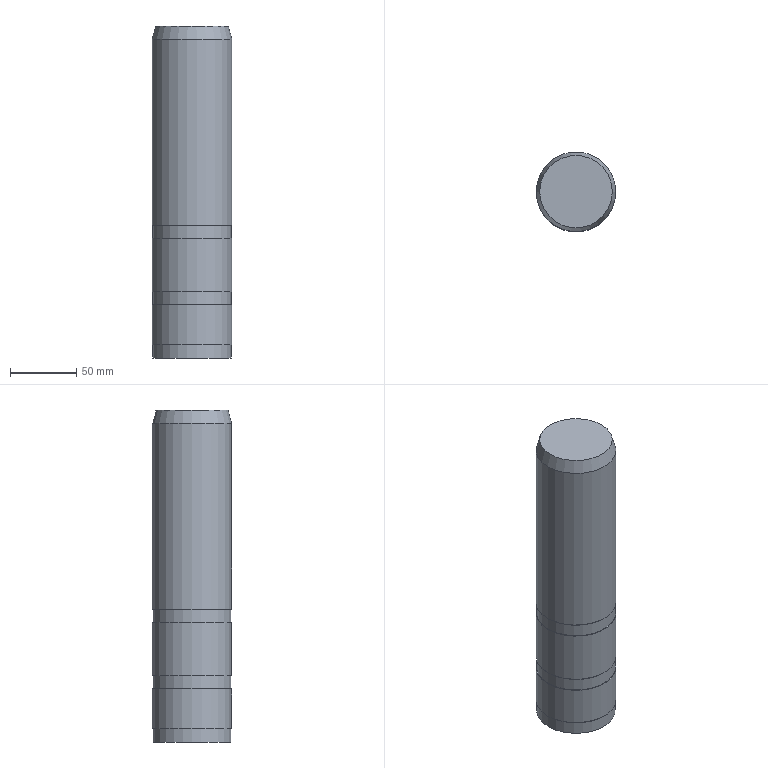Part | NX | features solid 2 | 1 solid | 14 faces | box 60 x 60 x 250 mm | volume 701604 mm3 | plane 7 | cylinder 6 | cone 1 | commonest cylinder face diameters 59 x3 60 x3
STEP:
#1=CARTESIAN_POINT('',(700.5,-25.,-150.));
#2=VERTEX_POINT('',#1);
#3=CARTESIAN_POINT('',(730.,-25.,-150.));
#4=DIRECTION('',(0.,0.,-1.));
#5=DIRECTION('',(-1.,0.,0.));
#6=AXIS2_PLACEMENT_3D('',#3,#4,#5);
#7=CIRCLE('',#6,29.5);
#8=EDGE_CURVE('',#2,#2,#7,.T.);
#9=ORIENTED_EDGE('',*,*,#8,.T.);
#10=EDGE_LOOP('',(#9));
#11=FACE_BOUND('',#10,.T.);
#12=CARTESIAN_POINT('',(700.5,-25.,-160.));
#13=VERTEX_POINT('',#12);
#14=CARTESIAN_POINT('',(730.,-25.,-160.));
#15=DIRECTION('',(0.,0.,-1.));
#16=DIRECTION('',(-1.,0.,0.));
#17=AXIS2_PLACEMENT_3D('',#14,#15,#16);
#18=CIRCLE('',#17,29.5);
#19=EDGE_CURVE('',#13,#13,#18,.T.);
#20=ORIENTED_EDGE('',*,*,#19,.F.);
#21=EDGE_LOOP('',(#20));
#22=FACE_BOUND('',#21,.T.);
#23=CARTESIAN_POINT('',(730.,-25.,-150.));
#24=DIRECTION('',(0.,0.,-1.));
#25=DIRECTION('',(1.,0.,0.));
#26=AXIS2_PLACEMENT_3D('',#23,#24,#25);
#27=CYLINDRICAL_SURFACE('',#26,29.5);
#28=ADVANCED_FACE('',(#11,#22),#27,.T.);
#29=CARTESIAN_POINT('',(700.,-25.,-150.));
#30=VERTEX_POINT('',#29);
#31=CARTESIAN_POINT('',(730.,-25.,-150.));
#32=DIRECTION('',(0.,0.,-1.));
#33=DIRECTION('',(-1.,0.,0.));
#34=AXIS2_PLACEMENT_3D('',#31,#32,#33);
#35=CIRCLE('',#34,30.);
#36=EDGE_CURVE('',#30,#30,#35,.T.);
#37=ORIENTED_EDGE('',*,*,#36,.T.);
#38=EDGE_LOOP('',(#37));
#39=FACE_BOUND('',#38,.T.);
#40=ORIENTED_EDGE('',*,*,#8,.F.);
#41=EDGE_LOOP('',(#40));
#42=FACE_BOUND('',#41,.T.);
#43=CARTESIAN_POINT('',(730.,-25.,-150.));
#44=DIRECTION('',(0.,0.,1.));
#45=DIRECTION('',(-1.,0.,0.));
#46=AXIS2_PLACEMENT_3D('',#43,#44,#45);
#47=PLANE('',#46);
#48=ADVANCED_FACE('',(#39,#42),#47,.F.);
#49=CARTESIAN_POINT('',(700.,-25.,-10.));
#50=VERTEX_POINT('',#49);
#51=CARTESIAN_POINT('',(730.,-25.,-10.));
#52=DIRECTION('',(0.,0.,-1.));
#53=DIRECTION('',(-1.,0.,0.));
#54=AXIS2_PLACEMENT_3D('',#51,#52,#53);
#55=CIRCLE('',#54,30.);
#56=EDGE_CURVE('',#50,#50,#55,.T.);
#57=ORIENTED_EDGE('',*,*,#56,.T.);
#58=EDGE_LOOP('',(#57));
#59=FACE_BOUND('',#58,.T.);
#60=ORIENTED_EDGE('',*,*,#36,.F.);
#61=EDGE_LOOP('',(#60));
#62=FACE_BOUND('',#61,.T.);
#63=CARTESIAN_POINT('',(730.,-25.,-10.));
#64=DIRECTION('',(0.,0.,-1.));
#65=DIRECTION('',(1.,0.,0.));
#66=AXIS2_PLACEMENT_3D('',#63,#64,#65);
#67=CYLINDRICAL_SURFACE('',#66,30.);
#68=ADVANCED_FACE('',(#59,#62),#67,.T.);
#69=CARTESIAN_POINT('',(702.679,-25.,0.));
#70=VERTEX_POINT('',#69);
#71=CARTESIAN_POINT('',(730.,-25.,0.));
#72=DIRECTION('',(0.,0.,-1.));
#73=DIRECTION('',(-1.,0.,0.));
#74=AXIS2_PLACEMENT_3D('',#71,#72,#73);
#75=CIRCLE('',#74,27.321);
#76=EDGE_CURVE('',#70,#70,#75,.T.);
#77=ORIENTED_EDGE('',*,*,#76,.T.);
#78=EDGE_LOOP('',(#77));
#79=FACE_BOUND('',#78,.T.);
#80=ORIENTED_EDGE('',*,*,#56,.F.);
#81=EDGE_LOOP('',(#80));
#82=FACE_BOUND('',#81,.T.);
#83=CARTESIAN_POINT('',(730.,-25.,-10.));
#84=DIRECTION('',(0.,0.,-1.));
#85=DIRECTION('',(-1.,0.,0.));
#86=AXIS2_PLACEMENT_3D('',#83,#84,#85);
#87=CONICAL_SURFACE('',#86,30.,0.2618);
#88=ADVANCED_FACE('',(#79,#82),#87,.T.);
#89=ORIENTED_EDGE('',*,*,#76,.F.);
#90=EDGE_LOOP('',(#89));
#91=FACE_BOUND('',#90,.T.);
#92=CARTESIAN_POINT('',(730.,-25.,0.));
#93=DIRECTION('',(0.,0.,1.));
#94=DIRECTION('',(-1.,0.,0.));
#95=AXIS2_PLACEMENT_3D('',#92,#93,#94);
#96=PLANE('',#95);
#97=ADVANCED_FACE('',(#91),#96,.T.);
#98=CARTESIAN_POINT('',(700.,-25.,-160.));
#99=VERTEX_POINT('',#98);
#100=CARTESIAN_POINT('',(730.,-25.,-160.));
#101=DIRECTION('',(0.,0.,-1.));
#102=DIRECTION('',(-1.,0.,0.));
#103=AXIS2_PLACEMENT_3D('',#100,#101,#102);
#104=CIRCLE('',#103,30.);
#105=EDGE_CURVE('',#99,#99,#104,.T.);
#106=ORIENTED_EDGE('',*,*,#105,.F.);
#107=EDGE_LOOP('',(#106));
#108=FACE_BOUND('',#107,.T.);
#109=ORIENTED_EDGE('',*,*,#19,.T.);
#110=EDGE_LOOP('',(#109));
#111=FACE_BOUND('',#110,.T.);
#112=CARTESIAN_POINT('',(730.,-25.,-160.));
#113=DIRECTION('',(0.,0.,1.));
#114=DIRECTION('',(-1.,0.,0.));
#115=AXIS2_PLACEMENT_3D('',#112,#113,#114);
#116=PLANE('',#115);
#117=ADVANCED_FACE('',(#108,#111),#116,.T.);
#118=CARTESIAN_POINT('',(700.,-25.,-200.));
#119=VERTEX_POINT('',#118);
#120=CARTESIAN_POINT('',(730.,-25.,-200.));
#121=DIRECTION('',(0.,0.,-1.));
#122=DIRECTION('',(-1.,0.,0.));
#123=AXIS2_PLACEMENT_3D('',#120,#121,#122);
#124=CIRCLE('',#123,30.);
#125=EDGE_CURVE('',#119,#119,#124,.T.);
#126=ORIENTED_EDGE('',*,*,#125,.F.);
#127=EDGE_LOOP('',(#126));
#128=FACE_BOUND('',#127,.T.);
#129=ORIENTED_EDGE('',*,*,#105,.T.);
#130=EDGE_LOOP('',(#129));
#131=FACE_BOUND('',#130,.T.);
#132=CARTESIAN_POINT('',(730.,-25.,-200.));
#133=DIRECTION('',(0.,0.,1.));
#134=DIRECTION('',(-1.,0.,0.));
#135=AXIS2_PLACEMENT_3D('',#132,#133,#134);
#136=CYLINDRICAL_SURFACE('',#135,30.);
#137=ADVANCED_FACE('',(#128,#131),#136,.T.);
#138=CARTESIAN_POINT('',(700.5,-25.,-200.));
#139=VERTEX_POINT('',#138);
#140=CARTESIAN_POINT('',(730.,-25.,-200.));
#141=DIRECTION('',(0.,0.,-1.));
#142=DIRECTION('',(-1.,0.,0.));
#143=AXIS2_PLACEMENT_3D('',#140,#141,#142);
#144=CIRCLE('',#143,29.5);
#145=EDGE_CURVE('',#139,#139,#144,.T.);
#146=ORIENTED_EDGE('',*,*,#145,.F.);
#147=EDGE_LOOP('',(#146));
#148=FACE_BOUND('',#147,.T.);
#149=ORIENTED_EDGE('',*,*,#125,.T.);
#150=EDGE_LOOP('',(#149));
#151=FACE_BOUND('',#150,.T.);
#152=CARTESIAN_POINT('',(730.,-25.,-200.));
#153=DIRECTION('',(0.,0.,1.));
#154=DIRECTION('',(-1.,0.,0.));
#155=AXIS2_PLACEMENT_3D('',#152,#153,#154);
#156=PLANE('',#155);
#157=ADVANCED_FACE('',(#148,#151),#156,.F.);
#158=CARTESIAN_POINT('',(700.5,-25.,-210.));
#159=VERTEX_POINT('',#158);
#160=CARTESIAN_POINT('',(730.,-25.,-210.));
#161=DIRECTION('',(0.,0.,-1.));
#162=DIRECTION('',(-1.,0.,0.));
#163=AXIS2_PLACEMENT_3D('',#160,#161,#162);
#164=CIRCLE('',#163,29.5);
#165=EDGE_CURVE('',#159,#159,#164,.F.);
#166=ORIENTED_EDGE('',*,*,#165,.T.);
#167=EDGE_LOOP('',(#166));
#168=FACE_BOUND('',#167,.T.);
#169=ORIENTED_EDGE('',*,*,#145,.T.);
#170=EDGE_LOOP('',(#169));
#171=FACE_BOUND('',#170,.T.);
#172=CARTESIAN_POINT('',(730.,-25.,-210.));
#173=DIRECTION('',(0.,0.,1.));
#174=DIRECTION('',(-1.,0.,0.));
#175=AXIS2_PLACEMENT_3D('',#172,#173,#174);
#176=CYLINDRICAL_SURFACE('',#175,29.5);
#177=ADVANCED_FACE('',(#168,#171),#176,.T.);
#178=CARTESIAN_POINT('',(700.,-25.,-240.));
#179=VERTEX_POINT('',#178);
#180=CARTESIAN_POINT('',(730.,-25.,-240.));
#181=DIRECTION('',(0.,0.,-1.));
#182=DIRECTION('',(-1.,0.,0.));
#183=AXIS2_PLACEMENT_3D('',#180,#181,#182);
#184=CIRCLE('',#183,30.);
#185=EDGE_CURVE('',#179,#179,#184,.T.);
#186=ORIENTED_EDGE('',*,*,#185,.F.);
#187=EDGE_LOOP('',(#186));
#188=FACE_BOUND('',#187,.T.);
#189=CARTESIAN_POINT('',(700.,-25.,-210.));
#190=VERTEX_POINT('',#189);
#191=CARTESIAN_POINT('',(730.,-25.,-210.));
#192=DIRECTION('',(0.,0.,-1.));
#193=DIRECTION('',(-1.,0.,0.));
#194=AXIS2_PLACEMENT_3D('',#191,#192,#193);
#195=CIRCLE('',#194,30.);
#196=EDGE_CURVE('',#190,#190,#195,.T.);
#197=ORIENTED_EDGE('',*,*,#196,.T.);
#198=EDGE_LOOP('',(#197));
#199=FACE_BOUND('',#198,.T.);
#200=CARTESIAN_POINT('',(730.,-25.,-240.));
#201=DIRECTION('',(0.,0.,1.));
#202=DIRECTION('',(-1.,0.,0.));
#203=AXIS2_PLACEMENT_3D('',#200,#201,#202);
#204=CYLINDRICAL_SURFACE('',#203,30.);
#205=ADVANCED_FACE('',(#188,#199),#204,.T.);
#206=CARTESIAN_POINT('',(700.5,-25.,-240.));
#207=VERTEX_POINT('',#206);
#208=CARTESIAN_POINT('',(730.,-25.,-240.));
#209=DIRECTION('',(0.,0.,-1.));
#210=DIRECTION('',(-1.,0.,0.));
#211=AXIS2_PLACEMENT_3D('',#208,#209,#210);
#212=CIRCLE('',#211,29.5);
#213=EDGE_CURVE('',#207,#207,#212,.T.);
#214=ORIENTED_EDGE('',*,*,#213,.F.);
#215=EDGE_LOOP('',(#214));
#216=FACE_BOUND('',#215,.T.);
#217=ORIENTED_EDGE('',*,*,#185,.T.);
#218=EDGE_LOOP('',(#217));
#219=FACE_BOUND('',#218,.T.);
#220=CARTESIAN_POINT('',(730.,-25.,-240.));
#221=DIRECTION('',(0.,0.,1.));
#222=DIRECTION('',(-1.,0.,0.));
#223=AXIS2_PLACEMENT_3D('',#220,#221,#222);
#224=PLANE('',#223);
#225=ADVANCED_FACE('',(#216,#219),#224,.F.);
#226=ORIENTED_EDGE('',*,*,#165,.F.);
#227=EDGE_LOOP('',(#226));
#228=FACE_BOUND('',#227,.T.);
#229=ORIENTED_EDGE('',*,*,#196,.F.);
#230=EDGE_LOOP('',(#229));
#231=FACE_BOUND('',#230,.T.);
#232=CARTESIAN_POINT('',(730.,-25.,-210.));
#233=DIRECTION('',(0.,0.,1.));
#234=DIRECTION('',(-1.,0.,0.));
#235=AXIS2_PLACEMENT_3D('',#232,#233,#234);
#236=PLANE('',#235);
#237=ADVANCED_FACE('',(#228,#231),#236,.T.);
#238=CARTESIAN_POINT('',(700.5,-25.,-250.));
#239=VERTEX_POINT('',#238);
#240=CARTESIAN_POINT('',(730.,-25.,-250.));
#241=DIRECTION('',(0.,0.,-1.));
#242=DIRECTION('',(-1.,0.,0.));
#243=AXIS2_PLACEMENT_3D('',#240,#241,#242);
#244=CIRCLE('',#243,29.5);
#245=EDGE_CURVE('',#239,#239,#244,.T.);
#246=ORIENTED_EDGE('',*,*,#245,.F.);
#247=EDGE_LOOP('',(#246));
#248=FACE_BOUND('',#247,.T.);
#249=ORIENTED_EDGE('',*,*,#213,.T.);
#250=EDGE_LOOP('',(#249));
#251=FACE_BOUND('',#250,.T.);
#252=CARTESIAN_POINT('',(730.,-25.,-250.));
#253=DIRECTION('',(0.,0.,1.));
#254=DIRECTION('',(-1.,0.,0.));
#255=AXIS2_PLACEMENT_3D('',#252,#253,#254);
#256=CYLINDRICAL_SURFACE('',#255,29.5);
#257=ADVANCED_FACE('',(#248,#251),#256,.T.);
#258=ORIENTED_EDGE('',*,*,#245,.T.);
#259=EDGE_LOOP('',(#258));
#260=FACE_BOUND('',#259,.T.);
#261=CARTESIAN_POINT('',(730.,-25.,-250.));
#262=DIRECTION('',(0.,0.,1.));
#263=DIRECTION('',(-1.,0.,0.));
#264=AXIS2_PLACEMENT_3D('',#261,#262,#263);
#265=PLANE('',#264);
#266=ADVANCED_FACE('',(#260),#265,.F.);
#267=CLOSED_SHELL('',(#28,#48,#68,#88,#97,#117,#137,#157,#177,#205,#225,#237,#257,#266));
#268=MANIFOLD_SOLID_BREP('',#267);
#269=(LENGTH_UNIT()NAMED_UNIT(*)SI_UNIT(.MILLI.,.METRE.));
#270=UNCERTAINTY_MEASURE_WITH_UNIT(LENGTH_MEASURE(0.00001),#269,'','');
#271=(NAMED_UNIT(*)PLANE_ANGLE_UNIT()SI_UNIT($,.RADIAN.));
#272=(NAMED_UNIT(*)SI_UNIT($,.STERADIAN.)SOLID_ANGLE_UNIT());
#273=(GEOMETRIC_REPRESENTATION_CONTEXT(3)GLOBAL_UNCERTAINTY_ASSIGNED_CONTEXT((#270))GLOBAL_UNIT_ASSIGNED_CONTEXT((#269,#271,#272))REPRESENTATION_CONTEXT('',''));
#274=ADVANCED_BREP_SHAPE_REPRESENTATION('',(#268),#273);